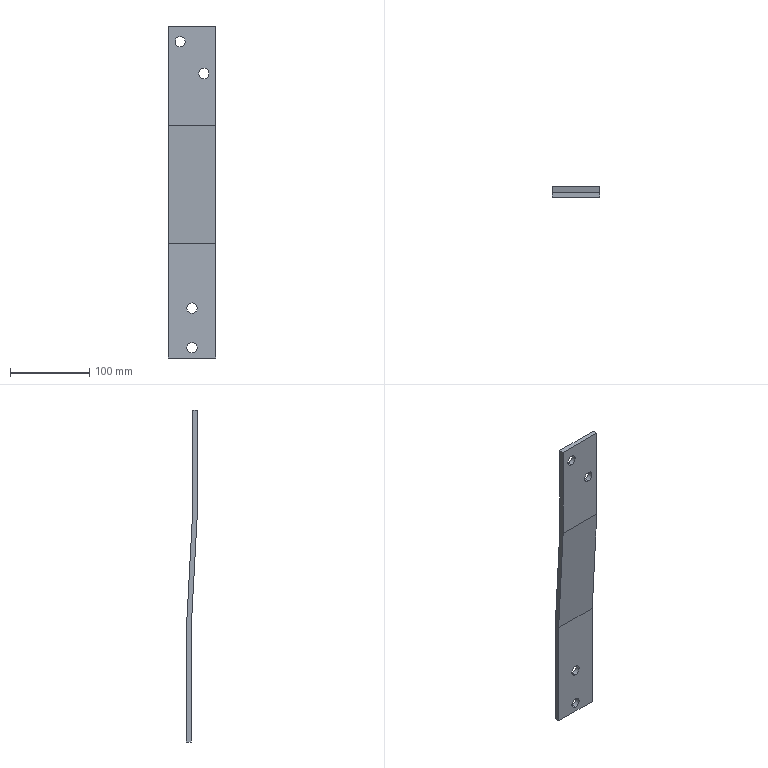Part | SolidWorks | features BaseBody 1 | 1 solid | 18 faces | box 60 x 14 x 419 mm | volume 147654 mm3 | plane 10 | cylinder 8 | commonest cylinder face diameters 13 x8
STEP:
#1=CARTESIAN_POINT('',(756.946,-3480.473,1580.471));
#2=VERTEX_POINT('',#1);
#3=CARTESIAN_POINT('',(756.946,-3480.473,1567.471));
#4=VERTEX_POINT('',#3);
#5=CARTESIAN_POINT('',(756.946,-3480.473,1573.971));
#6=DIRECTION('',(0.,-1.,0.));
#7=DIRECTION('',(0.,0.,-1.));
#8=AXIS2_PLACEMENT_3D('',#5,#6,#7);
#9=CIRCLE('',#8,6.5);
#10=EDGE_CURVE('',#2,#4,#9,.T.);
#11=ORIENTED_EDGE('',*,*,#10,.F.);
#12=CARTESIAN_POINT('',(756.946,-3486.473,1580.471));
#13=VERTEX_POINT('',#12);
#14=CARTESIAN_POINT('',(756.946,-3491.9,1580.471));
#15=DIRECTION('',(0.,-1.,0.));
#16=VECTOR('',#15,1000.);
#17=LINE('',#14,#16);
#18=EDGE_CURVE('',#2,#13,#17,.T.);
#19=ORIENTED_EDGE('',*,*,#18,.T.);
#20=CARTESIAN_POINT('',(756.946,-3486.473,1567.471));
#21=VERTEX_POINT('',#20);
#22=CARTESIAN_POINT('',(756.946,-3486.473,1573.971));
#23=DIRECTION('',(0.,1.,0.));
#24=DIRECTION('',(0.,0.,-1.));
#25=AXIS2_PLACEMENT_3D('',#22,#23,#24);
#26=CIRCLE('',#25,6.5);
#27=EDGE_CURVE('',#21,#13,#26,.T.);
#28=ORIENTED_EDGE('',*,*,#27,.F.);
#29=CARTESIAN_POINT('',(756.946,-3491.9,1567.471));
#30=DIRECTION('',(0.,-1.,0.));
#31=VECTOR('',#30,1000.);
#32=LINE('',#29,#31);
#33=EDGE_CURVE('',#4,#21,#32,.T.);
#34=ORIENTED_EDGE('',*,*,#33,.F.);
#35=EDGE_LOOP('',(#11,#19,#28,#34));
#36=FACE_OUTER_BOUND('',#35,.T.);
#37=CARTESIAN_POINT('',(756.946,-3491.9,1573.971));
#38=DIRECTION('',(0.,-1.,0.));
#39=DIRECTION('',(0.,0.,-1.));
#40=AXIS2_PLACEMENT_3D('',#37,#38,#39);
#41=CYLINDRICAL_SURFACE('',#40,6.5);
#42=ADVANCED_FACE('',(#36),#41,.F.);
#43=CARTESIAN_POINT('',(756.946,-3480.473,1530.471));
#44=VERTEX_POINT('',#43);
#45=CARTESIAN_POINT('',(756.946,-3480.473,1517.471));
#46=VERTEX_POINT('',#45);
#47=CARTESIAN_POINT('',(756.946,-3480.473,1523.971));
#48=DIRECTION('',(0.,-1.,0.));
#49=DIRECTION('',(0.,0.,-1.));
#50=AXIS2_PLACEMENT_3D('',#47,#48,#49);
#51=CIRCLE('',#50,6.5);
#52=EDGE_CURVE('',#44,#46,#51,.T.);
#53=ORIENTED_EDGE('',*,*,#52,.F.);
#54=CARTESIAN_POINT('',(756.946,-3486.473,1530.471));
#55=VERTEX_POINT('',#54);
#56=CARTESIAN_POINT('',(756.946,-3491.9,1530.471));
#57=DIRECTION('',(0.,-1.,0.));
#58=VECTOR('',#57,1000.);
#59=LINE('',#56,#58);
#60=EDGE_CURVE('',#44,#55,#59,.T.);
#61=ORIENTED_EDGE('',*,*,#60,.T.);
#62=CARTESIAN_POINT('',(756.946,-3486.473,1517.471));
#63=VERTEX_POINT('',#62);
#64=CARTESIAN_POINT('',(756.946,-3486.473,1523.971));
#65=DIRECTION('',(0.,1.,0.));
#66=DIRECTION('',(0.,0.,-1.));
#67=AXIS2_PLACEMENT_3D('',#64,#65,#66);
#68=CIRCLE('',#67,6.5);
#69=EDGE_CURVE('',#63,#55,#68,.T.);
#70=ORIENTED_EDGE('',*,*,#69,.F.);
#71=CARTESIAN_POINT('',(756.946,-3491.9,1517.471));
#72=DIRECTION('',(0.,-1.,0.));
#73=VECTOR('',#72,1000.);
#74=LINE('',#71,#73);
#75=EDGE_CURVE('',#46,#63,#74,.T.);
#76=ORIENTED_EDGE('',*,*,#75,.F.);
#77=EDGE_LOOP('',(#53,#61,#70,#76));
#78=FACE_OUTER_BOUND('',#77,.T.);
#79=CARTESIAN_POINT('',(756.946,-3491.9,1523.971));
#80=DIRECTION('',(0.,-1.,0.));
#81=DIRECTION('',(0.,0.,-1.));
#82=AXIS2_PLACEMENT_3D('',#79,#80,#81);
#83=CYLINDRICAL_SURFACE('',#82,6.5);
#84=ADVANCED_FACE('',(#78),#83,.F.);
#85=CARTESIAN_POINT('',(741.946,-3488.473,1916.471));
#86=VERTEX_POINT('',#85);
#87=CARTESIAN_POINT('',(741.946,-3488.473,1903.471));
#88=VERTEX_POINT('',#87);
#89=CARTESIAN_POINT('',(741.946,-3488.473,1909.971));
#90=DIRECTION('',(0.,-1.,0.));
#91=DIRECTION('',(0.,0.,-1.));
#92=AXIS2_PLACEMENT_3D('',#89,#90,#91);
#93=CIRCLE('',#92,6.5);
#94=EDGE_CURVE('',#86,#88,#93,.T.);
#95=ORIENTED_EDGE('',*,*,#94,.F.);
#96=CARTESIAN_POINT('',(741.946,-3494.473,1916.471));
#97=VERTEX_POINT('',#96);
#98=CARTESIAN_POINT('',(741.946,-3489.856,1916.471));
#99=DIRECTION('',(0.,-1.,0.));
#100=VECTOR('',#99,1000.);
#101=LINE('',#98,#100);
#102=EDGE_CURVE('',#86,#97,#101,.T.);
#103=ORIENTED_EDGE('',*,*,#102,.T.);
#104=CARTESIAN_POINT('',(741.946,-3494.473,1903.471));
#105=VERTEX_POINT('',#104);
#106=CARTESIAN_POINT('',(741.946,-3494.473,1909.971));
#107=DIRECTION('',(0.,1.,0.));
#108=DIRECTION('',(0.,0.,-1.));
#109=AXIS2_PLACEMENT_3D('',#106,#107,#108);
#110=CIRCLE('',#109,6.5);
#111=EDGE_CURVE('',#105,#97,#110,.T.);
#112=ORIENTED_EDGE('',*,*,#111,.F.);
#113=CARTESIAN_POINT('',(741.946,-3489.856,1903.471));
#114=DIRECTION('',(0.,-1.,0.));
#115=VECTOR('',#114,1000.);
#116=LINE('',#113,#115);
#117=EDGE_CURVE('',#88,#105,#116,.T.);
#118=ORIENTED_EDGE('',*,*,#117,.F.);
#119=EDGE_LOOP('',(#95,#103,#112,#118));
#120=FACE_OUTER_BOUND('',#119,.T.);
#121=CARTESIAN_POINT('',(741.946,-3489.856,1909.971));
#122=DIRECTION('',(0.,-1.,0.));
#123=DIRECTION('',(0.,0.,-1.));
#124=AXIS2_PLACEMENT_3D('',#121,#122,#123);
#125=CYLINDRICAL_SURFACE('',#124,6.5);
#126=ADVANCED_FACE('',(#120),#125,.F.);
#127=CARTESIAN_POINT('',(771.946,-3488.473,1876.471));
#128=VERTEX_POINT('',#127);
#129=CARTESIAN_POINT('',(771.946,-3488.473,1863.471));
#130=VERTEX_POINT('',#129);
#131=CARTESIAN_POINT('',(771.946,-3488.473,1869.971));
#132=DIRECTION('',(0.,-1.,0.));
#133=DIRECTION('',(0.,0.,-1.));
#134=AXIS2_PLACEMENT_3D('',#131,#132,#133);
#135=CIRCLE('',#134,6.5);
#136=EDGE_CURVE('',#128,#130,#135,.T.);
#137=ORIENTED_EDGE('',*,*,#136,.F.);
#138=CARTESIAN_POINT('',(771.946,-3494.473,1876.471));
#139=VERTEX_POINT('',#138);
#140=CARTESIAN_POINT('',(771.946,-3487.265,1876.471));
#141=DIRECTION('',(0.,-1.,0.));
#142=VECTOR('',#141,1000.);
#143=LINE('',#140,#142);
#144=EDGE_CURVE('',#128,#139,#143,.T.);
#145=ORIENTED_EDGE('',*,*,#144,.T.);
#146=CARTESIAN_POINT('',(771.946,-3494.473,1863.471));
#147=VERTEX_POINT('',#146);
#148=CARTESIAN_POINT('',(771.946,-3494.473,1869.971));
#149=DIRECTION('',(0.,1.,0.));
#150=DIRECTION('',(0.,0.,-1.));
#151=AXIS2_PLACEMENT_3D('',#148,#149,#150);
#152=CIRCLE('',#151,6.5);
#153=EDGE_CURVE('',#147,#139,#152,.T.);
#154=ORIENTED_EDGE('',*,*,#153,.F.);
#155=CARTESIAN_POINT('',(771.946,-3487.265,1863.471));
#156=DIRECTION('',(0.,-1.,0.));
#157=VECTOR('',#156,1000.);
#158=LINE('',#155,#157);
#159=EDGE_CURVE('',#130,#147,#158,.T.);
#160=ORIENTED_EDGE('',*,*,#159,.F.);
#161=EDGE_LOOP('',(#137,#145,#154,#160));
#162=FACE_OUTER_BOUND('',#161,.T.);
#163=CARTESIAN_POINT('',(771.946,-3487.265,1869.971));
#164=DIRECTION('',(0.,-1.,0.));
#165=DIRECTION('',(0.,0.,-1.));
#166=AXIS2_PLACEMENT_3D('',#163,#164,#165);
#167=CYLINDRICAL_SURFACE('',#166,6.5);
#168=ADVANCED_FACE('',(#162),#167,.F.);
#169=CARTESIAN_POINT('',(786.946,-3488.473,1804.971));
#170=VERTEX_POINT('',#169);
#171=CARTESIAN_POINT('',(786.946,-3480.473,1654.971));
#172=VERTEX_POINT('',#171);
#173=CARTESIAN_POINT('',(786.946,-3480.473,1654.971));
#174=DIRECTION('',(0.,0.05326,-0.9986));
#175=VECTOR('',#174,1000.);
#176=LINE('',#173,#175);
#177=EDGE_CURVE('',#170,#172,#176,.T.);
#178=ORIENTED_EDGE('',*,*,#177,.T.);
#179=CARTESIAN_POINT('',(726.946,-3480.473,1654.971));
#180=VERTEX_POINT('',#179);
#181=CARTESIAN_POINT('',(786.946,-3480.473,1654.971));
#182=DIRECTION('',(-1.,0.,0.));
#183=VECTOR('',#182,1000.);
#184=LINE('',#181,#183);
#185=EDGE_CURVE('',#172,#180,#184,.T.);
#186=ORIENTED_EDGE('',*,*,#185,.T.);
#187=CARTESIAN_POINT('',(726.946,-3488.473,1804.971));
#188=VERTEX_POINT('',#187);
#189=CARTESIAN_POINT('',(726.946,-3480.473,1654.971));
#190=DIRECTION('',(0.,-0.05326,0.9986));
#191=VECTOR('',#190,1000.);
#192=LINE('',#189,#191);
#193=EDGE_CURVE('',#180,#188,#192,.T.);
#194=ORIENTED_EDGE('',*,*,#193,.T.);
#195=CARTESIAN_POINT('',(786.946,-3488.473,1804.971));
#196=DIRECTION('',(1.,0.,0.));
#197=VECTOR('',#196,1000.);
#198=LINE('',#195,#197);
#199=EDGE_CURVE('',#188,#170,#198,.T.);
#200=ORIENTED_EDGE('',*,*,#199,.T.);
#201=EDGE_LOOP('',(#178,#186,#194,#200));
#202=FACE_OUTER_BOUND('',#201,.T.);
#203=CARTESIAN_POINT('',(786.946,-3480.473,1654.971));
#204=DIRECTION('',(0.,0.9986,0.05326));
#205=DIRECTION('',(0.,-0.05326,0.9986));
#206=AXIS2_PLACEMENT_3D('',#203,#204,#205);
#207=PLANE('',#206);
#208=ADVANCED_FACE('',(#202),#207,.T.);
#209=CARTESIAN_POINT('',(786.946,-3480.473,1510.971));
#210=VERTEX_POINT('',#209);
#211=CARTESIAN_POINT('',(786.946,-3480.473,1510.971));
#212=DIRECTION('',(0.,0.,-1.));
#213=VECTOR('',#212,1000.);
#214=LINE('',#211,#213);
#215=EDGE_CURVE('',#172,#210,#214,.T.);
#216=ORIENTED_EDGE('',*,*,#215,.T.);
#217=CARTESIAN_POINT('',(726.946,-3480.473,1510.971));
#218=VERTEX_POINT('',#217);
#219=CARTESIAN_POINT('',(786.946,-3480.473,1510.971));
#220=DIRECTION('',(-1.,0.,0.));
#221=VECTOR('',#220,1000.);
#222=LINE('',#219,#221);
#223=EDGE_CURVE('',#210,#218,#222,.T.);
#224=ORIENTED_EDGE('',*,*,#223,.T.);
#225=CARTESIAN_POINT('',(726.946,-3480.473,1510.971));
#226=DIRECTION('',(0.,0.,1.));
#227=VECTOR('',#226,1000.);
#228=LINE('',#225,#227);
#229=EDGE_CURVE('',#218,#180,#228,.T.);
#230=ORIENTED_EDGE('',*,*,#229,.T.);
#231=ORIENTED_EDGE('',*,*,#185,.F.);
#232=EDGE_LOOP('',(#216,#224,#230,#231));
#233=FACE_OUTER_BOUND('',#232,.T.);
#234=CARTESIAN_POINT('',(756.946,-3480.473,1573.971));
#235=DIRECTION('',(0.,-1.,0.));
#236=DIRECTION('',(0.,0.,-1.));
#237=AXIS2_PLACEMENT_3D('',#234,#235,#236);
#238=CIRCLE('',#237,6.5);
#239=EDGE_CURVE('',#4,#2,#238,.T.);
#240=ORIENTED_EDGE('',*,*,#239,.T.);
#241=ORIENTED_EDGE('',*,*,#10,.T.);
#242=EDGE_LOOP('',(#240,#241));
#243=FACE_BOUND('',#242,.T.);
#244=CARTESIAN_POINT('',(756.946,-3480.473,1523.971));
#245=DIRECTION('',(0.,-1.,0.));
#246=DIRECTION('',(0.,0.,-1.));
#247=AXIS2_PLACEMENT_3D('',#244,#245,#246);
#248=CIRCLE('',#247,6.5);
#249=EDGE_CURVE('',#46,#44,#248,.T.);
#250=ORIENTED_EDGE('',*,*,#249,.T.);
#251=ORIENTED_EDGE('',*,*,#52,.T.);
#252=EDGE_LOOP('',(#250,#251));
#253=FACE_BOUND('',#252,.T.);
#254=CARTESIAN_POINT('',(786.946,-3480.473,1510.971));
#255=DIRECTION('',(0.,1.,0.));
#256=DIRECTION('',(0.,0.,1.));
#257=AXIS2_PLACEMENT_3D('',#254,#255,#256);
#258=PLANE('',#257);
#259=ADVANCED_FACE('',(#233,#243,#253),#258,.T.);
#260=CARTESIAN_POINT('',(786.946,-3494.473,1804.971));
#261=VERTEX_POINT('',#260);
#262=CARTESIAN_POINT('',(786.946,-3486.473,1654.971));
#263=VERTEX_POINT('',#262);
#264=CARTESIAN_POINT('',(786.946,-3494.473,1804.971));
#265=DIRECTION('',(0.,0.05326,-0.9986));
#266=VECTOR('',#265,1000.);
#267=LINE('',#264,#266);
#268=EDGE_CURVE('',#261,#263,#267,.T.);
#269=ORIENTED_EDGE('',*,*,#268,.T.);
#270=CARTESIAN_POINT('',(786.946,-3486.473,1510.971));
#271=VERTEX_POINT('',#270);
#272=CARTESIAN_POINT('',(786.946,-3486.473,1707.983));
#273=DIRECTION('',(0.,0.,-1.));
#274=VECTOR('',#273,1000.);
#275=LINE('',#272,#274);
#276=EDGE_CURVE('',#263,#271,#275,.T.);
#277=ORIENTED_EDGE('',*,*,#276,.T.);
#278=CARTESIAN_POINT('',(786.946,-3487.033,1510.971));
#279=DIRECTION('',(0.,1.,0.));
#280=VECTOR('',#279,1000.);
#281=LINE('',#278,#280);
#282=EDGE_CURVE('',#271,#210,#281,.T.);
#283=ORIENTED_EDGE('',*,*,#282,.T.);
#284=ORIENTED_EDGE('',*,*,#215,.F.);
#285=ORIENTED_EDGE('',*,*,#177,.F.);
#286=CARTESIAN_POINT('',(786.946,-3488.473,1929.971));
#287=VERTEX_POINT('',#286);
#288=CARTESIAN_POINT('',(786.946,-3488.473,1707.983));
#289=DIRECTION('',(0.,0.,1.));
#290=VECTOR('',#289,1000.);
#291=LINE('',#288,#290);
#292=EDGE_CURVE('',#170,#287,#291,.T.);
#293=ORIENTED_EDGE('',*,*,#292,.T.);
#294=CARTESIAN_POINT('',(786.946,-3494.473,1929.971));
#295=VERTEX_POINT('',#294);
#296=CARTESIAN_POINT('',(786.946,-3487.033,1929.971));
#297=DIRECTION('',(0.,-1.,0.));
#298=VECTOR('',#297,1000.);
#299=LINE('',#296,#298);
#300=EDGE_CURVE('',#287,#295,#299,.T.);
#301=ORIENTED_EDGE('',*,*,#300,.T.);
#302=CARTESIAN_POINT('',(786.946,-3494.473,1707.983));
#303=DIRECTION('',(0.,0.,-1.));
#304=VECTOR('',#303,1000.);
#305=LINE('',#302,#304);
#306=EDGE_CURVE('',#295,#261,#305,.T.);
#307=ORIENTED_EDGE('',*,*,#306,.T.);
#308=EDGE_LOOP('',(#269,#277,#283,#284,#285,#293,#301,#307));
#309=FACE_OUTER_BOUND('',#308,.T.);
#310=CARTESIAN_POINT('',(786.946,-3487.033,1707.983));
#311=DIRECTION('',(1.,0.,0.));
#312=DIRECTION('',(0.,0.,-1.));
#313=AXIS2_PLACEMENT_3D('',#310,#311,#312);
#314=PLANE('',#313);
#315=ADVANCED_FACE('',(#309),#314,.T.);
#316=ORIENTED_EDGE('',*,*,#292,.F.);
#317=ORIENTED_EDGE('',*,*,#199,.F.);
#318=CARTESIAN_POINT('',(726.946,-3488.473,1929.971));
#319=VERTEX_POINT('',#318);
#320=CARTESIAN_POINT('',(726.946,-3488.473,1804.971));
#321=DIRECTION('',(0.,0.,1.));
#322=VECTOR('',#321,1000.);
#323=LINE('',#320,#322);
#324=EDGE_CURVE('',#188,#319,#323,.T.);
#325=ORIENTED_EDGE('',*,*,#324,.T.);
#326=CARTESIAN_POINT('',(786.946,-3488.473,1929.971));
#327=DIRECTION('',(1.,0.,0.));
#328=VECTOR('',#327,1000.);
#329=LINE('',#326,#328);
#330=EDGE_CURVE('',#319,#287,#329,.T.);
#331=ORIENTED_EDGE('',*,*,#330,.T.);
#332=EDGE_LOOP('',(#316,#317,#325,#331));
#333=FACE_OUTER_BOUND('',#332,.T.);
#334=CARTESIAN_POINT('',(741.946,-3488.473,1909.971));
#335=DIRECTION('',(0.,-1.,0.));
#336=DIRECTION('',(0.,0.,-1.));
#337=AXIS2_PLACEMENT_3D('',#334,#335,#336);
#338=CIRCLE('',#337,6.5);
#339=EDGE_CURVE('',#88,#86,#338,.T.);
#340=ORIENTED_EDGE('',*,*,#339,.T.);
#341=ORIENTED_EDGE('',*,*,#94,.T.);
#342=EDGE_LOOP('',(#340,#341));
#343=FACE_BOUND('',#342,.T.);
#344=CARTESIAN_POINT('',(771.946,-3488.473,1869.971));
#345=DIRECTION('',(0.,-1.,0.));
#346=DIRECTION('',(0.,0.,-1.));
#347=AXIS2_PLACEMENT_3D('',#344,#345,#346);
#348=CIRCLE('',#347,6.5);
#349=EDGE_CURVE('',#130,#128,#348,.T.);
#350=ORIENTED_EDGE('',*,*,#349,.T.);
#351=ORIENTED_EDGE('',*,*,#136,.T.);
#352=EDGE_LOOP('',(#350,#351));
#353=FACE_BOUND('',#352,.T.);
#354=CARTESIAN_POINT('',(786.946,-3488.473,1804.971));
#355=DIRECTION('',(0.,1.,0.));
#356=DIRECTION('',(0.,0.,1.));
#357=AXIS2_PLACEMENT_3D('',#354,#355,#356);
#358=PLANE('',#357);
#359=ADVANCED_FACE('',(#333,#343,#353),#358,.T.);
#360=CARTESIAN_POINT('',(726.946,-3486.473,1510.971));
#361=VERTEX_POINT('',#360);
#362=CARTESIAN_POINT('',(726.946,-3487.033,1510.971));
#363=DIRECTION('',(0.,1.,0.));
#364=VECTOR('',#363,1000.);
#365=LINE('',#362,#364);
#366=EDGE_CURVE('',#361,#218,#365,.T.);
#367=ORIENTED_EDGE('',*,*,#366,.F.);
#368=CARTESIAN_POINT('',(726.946,-3486.473,1654.971));
#369=VERTEX_POINT('',#368);
#370=CARTESIAN_POINT('',(726.946,-3486.473,1707.983));
#371=DIRECTION('',(0.,0.,-1.));
#372=VECTOR('',#371,1000.);
#373=LINE('',#370,#372);
#374=EDGE_CURVE('',#369,#361,#373,.T.);
#375=ORIENTED_EDGE('',*,*,#374,.F.);
#376=CARTESIAN_POINT('',(726.946,-3494.473,1804.971));
#377=VERTEX_POINT('',#376);
#378=CARTESIAN_POINT('',(726.946,-3494.473,1804.971));
#379=DIRECTION('',(0.,0.05326,-0.9986));
#380=VECTOR('',#379,1000.);
#381=LINE('',#378,#380);
#382=EDGE_CURVE('',#377,#369,#381,.T.);
#383=ORIENTED_EDGE('',*,*,#382,.F.);
#384=CARTESIAN_POINT('',(726.946,-3494.473,1929.971));
#385=VERTEX_POINT('',#384);
#386=CARTESIAN_POINT('',(726.946,-3494.473,1707.983));
#387=DIRECTION('',(0.,0.,-1.));
#388=VECTOR('',#387,1000.);
#389=LINE('',#386,#388);
#390=EDGE_CURVE('',#385,#377,#389,.T.);
#391=ORIENTED_EDGE('',*,*,#390,.F.);
#392=CARTESIAN_POINT('',(726.946,-3487.033,1929.971));
#393=DIRECTION('',(0.,-1.,0.));
#394=VECTOR('',#393,1000.);
#395=LINE('',#392,#394);
#396=EDGE_CURVE('',#319,#385,#395,.T.);
#397=ORIENTED_EDGE('',*,*,#396,.F.);
#398=ORIENTED_EDGE('',*,*,#324,.F.);
#399=ORIENTED_EDGE('',*,*,#193,.F.);
#400=ORIENTED_EDGE('',*,*,#229,.F.);
#401=EDGE_LOOP('',(#367,#375,#383,#391,#397,#398,#399,#400));
#402=FACE_OUTER_BOUND('',#401,.T.);
#403=CARTESIAN_POINT('',(726.946,-3487.033,1707.983));
#404=DIRECTION('',(1.,0.,0.));
#405=DIRECTION('',(0.,0.,-1.));
#406=AXIS2_PLACEMENT_3D('',#403,#404,#405);
#407=PLANE('',#406);
#408=ADVANCED_FACE('',(#402),#407,.F.);
#409=ORIENTED_EDGE('',*,*,#282,.F.);
#410=CARTESIAN_POINT('',(786.946,-3486.473,1510.971));
#411=DIRECTION('',(-1.,0.,0.));
#412=VECTOR('',#411,1000.);
#413=LINE('',#410,#412);
#414=EDGE_CURVE('',#271,#361,#413,.T.);
#415=ORIENTED_EDGE('',*,*,#414,.T.);
#416=ORIENTED_EDGE('',*,*,#366,.T.);
#417=ORIENTED_EDGE('',*,*,#223,.F.);
#418=EDGE_LOOP('',(#409,#415,#416,#417));
#419=FACE_OUTER_BOUND('',#418,.T.);
#420=CARTESIAN_POINT('',(786.946,-3486.473,1510.971));
#421=DIRECTION('',(0.,0.,-1.));
#422=DIRECTION('',(-1.,0.,0.));
#423=AXIS2_PLACEMENT_3D('',#420,#421,#422);
#424=PLANE('',#423);
#425=ADVANCED_FACE('',(#419),#424,.T.);
#426=ORIENTED_EDGE('',*,*,#18,.F.);
#427=ORIENTED_EDGE('',*,*,#239,.F.);
#428=ORIENTED_EDGE('',*,*,#33,.T.);
#429=CARTESIAN_POINT('',(756.946,-3486.473,1573.971));
#430=DIRECTION('',(0.,1.,0.));
#431=DIRECTION('',(0.,0.,-1.));
#432=AXIS2_PLACEMENT_3D('',#429,#430,#431);
#433=CIRCLE('',#432,6.5);
#434=EDGE_CURVE('',#13,#21,#433,.T.);
#435=ORIENTED_EDGE('',*,*,#434,.F.);
#436=EDGE_LOOP('',(#426,#427,#428,#435));
#437=FACE_OUTER_BOUND('',#436,.T.);
#438=CARTESIAN_POINT('',(756.946,-3491.9,1573.971));
#439=DIRECTION('',(0.,-1.,0.));
#440=DIRECTION('',(0.,0.,-1.));
#441=AXIS2_PLACEMENT_3D('',#438,#439,#440);
#442=CYLINDRICAL_SURFACE('',#441,6.5);
#443=ADVANCED_FACE('',(#437),#442,.F.);
#444=ORIENTED_EDGE('',*,*,#60,.F.);
#445=ORIENTED_EDGE('',*,*,#249,.F.);
#446=ORIENTED_EDGE('',*,*,#75,.T.);
#447=CARTESIAN_POINT('',(756.946,-3486.473,1523.971));
#448=DIRECTION('',(0.,1.,0.));
#449=DIRECTION('',(0.,0.,-1.));
#450=AXIS2_PLACEMENT_3D('',#447,#448,#449);
#451=CIRCLE('',#450,6.5);
#452=EDGE_CURVE('',#55,#63,#451,.T.);
#453=ORIENTED_EDGE('',*,*,#452,.F.);
#454=EDGE_LOOP('',(#444,#445,#446,#453));
#455=FACE_OUTER_BOUND('',#454,.T.);
#456=CARTESIAN_POINT('',(756.946,-3491.9,1523.971));
#457=DIRECTION('',(0.,-1.,0.));
#458=DIRECTION('',(0.,0.,-1.));
#459=AXIS2_PLACEMENT_3D('',#456,#457,#458);
#460=CYLINDRICAL_SURFACE('',#459,6.5);
#461=ADVANCED_FACE('',(#455),#460,.F.);
#462=ORIENTED_EDGE('',*,*,#276,.F.);
#463=CARTESIAN_POINT('',(786.946,-3486.473,1654.971));
#464=DIRECTION('',(-1.,0.,0.));
#465=VECTOR('',#464,1000.);
#466=LINE('',#463,#465);
#467=EDGE_CURVE('',#263,#369,#466,.T.);
#468=ORIENTED_EDGE('',*,*,#467,.T.);
#469=ORIENTED_EDGE('',*,*,#374,.T.);
#470=ORIENTED_EDGE('',*,*,#414,.F.);
#471=EDGE_LOOP('',(#462,#468,#469,#470));
#472=FACE_OUTER_BOUND('',#471,.T.);
#473=ORIENTED_EDGE('',*,*,#27,.T.);
#474=ORIENTED_EDGE('',*,*,#434,.T.);
#475=EDGE_LOOP('',(#473,#474));
#476=FACE_BOUND('',#475,.T.);
#477=ORIENTED_EDGE('',*,*,#69,.T.);
#478=ORIENTED_EDGE('',*,*,#452,.T.);
#479=EDGE_LOOP('',(#477,#478));
#480=FACE_BOUND('',#479,.T.);
#481=CARTESIAN_POINT('',(786.946,-3486.473,1654.971));
#482=DIRECTION('',(0.,-1.,0.));
#483=DIRECTION('',(0.,0.,-1.));
#484=AXIS2_PLACEMENT_3D('',#481,#482,#483);
#485=PLANE('',#484);
#486=ADVANCED_FACE('',(#472,#476,#480),#485,.T.);
#487=ORIENTED_EDGE('',*,*,#268,.F.);
#488=CARTESIAN_POINT('',(786.946,-3494.473,1804.971));
#489=DIRECTION('',(-1.,0.,0.));
#490=VECTOR('',#489,1000.);
#491=LINE('',#488,#490);
#492=EDGE_CURVE('',#261,#377,#491,.T.);
#493=ORIENTED_EDGE('',*,*,#492,.T.);
#494=ORIENTED_EDGE('',*,*,#382,.T.);
#495=ORIENTED_EDGE('',*,*,#467,.F.);
#496=EDGE_LOOP('',(#487,#493,#494,#495));
#497=FACE_OUTER_BOUND('',#496,.T.);
#498=CARTESIAN_POINT('',(786.946,-3494.473,1804.971));
#499=DIRECTION('',(0.,-0.9986,-0.05326));
#500=DIRECTION('',(0.,0.05326,-0.9986));
#501=AXIS2_PLACEMENT_3D('',#498,#499,#500);
#502=PLANE('',#501);
#503=ADVANCED_FACE('',(#497),#502,.T.);
#504=ORIENTED_EDGE('',*,*,#306,.F.);
#505=CARTESIAN_POINT('',(786.946,-3494.473,1929.971));
#506=DIRECTION('',(-1.,0.,0.));
#507=VECTOR('',#506,1000.);
#508=LINE('',#505,#507);
#509=EDGE_CURVE('',#295,#385,#508,.T.);
#510=ORIENTED_EDGE('',*,*,#509,.T.);
#511=ORIENTED_EDGE('',*,*,#390,.T.);
#512=ORIENTED_EDGE('',*,*,#492,.F.);
#513=EDGE_LOOP('',(#504,#510,#511,#512));
#514=FACE_OUTER_BOUND('',#513,.T.);
#515=ORIENTED_EDGE('',*,*,#111,.T.);
#516=CARTESIAN_POINT('',(741.946,-3494.473,1909.971));
#517=DIRECTION('',(0.,1.,0.));
#518=DIRECTION('',(0.,0.,-1.));
#519=AXIS2_PLACEMENT_3D('',#516,#517,#518);
#520=CIRCLE('',#519,6.5);
#521=EDGE_CURVE('',#97,#105,#520,.T.);
#522=ORIENTED_EDGE('',*,*,#521,.T.);
#523=EDGE_LOOP('',(#515,#522));
#524=FACE_BOUND('',#523,.T.);
#525=ORIENTED_EDGE('',*,*,#153,.T.);
#526=CARTESIAN_POINT('',(771.946,-3494.473,1869.971));
#527=DIRECTION('',(0.,1.,0.));
#528=DIRECTION('',(0.,0.,-1.));
#529=AXIS2_PLACEMENT_3D('',#526,#527,#528);
#530=CIRCLE('',#529,6.5);
#531=EDGE_CURVE('',#139,#147,#530,.T.);
#532=ORIENTED_EDGE('',*,*,#531,.T.);
#533=EDGE_LOOP('',(#525,#532));
#534=FACE_BOUND('',#533,.T.);
#535=CARTESIAN_POINT('',(786.946,-3494.473,1904.971));
#536=DIRECTION('',(0.,-1.,0.));
#537=DIRECTION('',(0.,0.,-1.));
#538=AXIS2_PLACEMENT_3D('',#535,#536,#537);
#539=PLANE('',#538);
#540=ADVANCED_FACE('',(#514,#524,#534),#539,.T.);
#541=ORIENTED_EDGE('',*,*,#300,.F.);
#542=ORIENTED_EDGE('',*,*,#330,.F.);
#543=ORIENTED_EDGE('',*,*,#396,.T.);
#544=ORIENTED_EDGE('',*,*,#509,.F.);
#545=EDGE_LOOP('',(#541,#542,#543,#544));
#546=FACE_OUTER_BOUND('',#545,.T.);
#547=CARTESIAN_POINT('',(786.946,-3488.473,1929.971));
#548=DIRECTION('',(0.,0.,1.));
#549=DIRECTION('',(1.,0.,0.));
#550=AXIS2_PLACEMENT_3D('',#547,#548,#549);
#551=PLANE('',#550);
#552=ADVANCED_FACE('',(#546),#551,.T.);
#553=ORIENTED_EDGE('',*,*,#102,.F.);
#554=ORIENTED_EDGE('',*,*,#339,.F.);
#555=ORIENTED_EDGE('',*,*,#117,.T.);
#556=ORIENTED_EDGE('',*,*,#521,.F.);
#557=EDGE_LOOP('',(#553,#554,#555,#556));
#558=FACE_OUTER_BOUND('',#557,.T.);
#559=CARTESIAN_POINT('',(741.946,-3489.856,1909.971));
#560=DIRECTION('',(0.,-1.,0.));
#561=DIRECTION('',(0.,0.,-1.));
#562=AXIS2_PLACEMENT_3D('',#559,#560,#561);
#563=CYLINDRICAL_SURFACE('',#562,6.5);
#564=ADVANCED_FACE('',(#558),#563,.F.);
#565=ORIENTED_EDGE('',*,*,#144,.F.);
#566=ORIENTED_EDGE('',*,*,#349,.F.);
#567=ORIENTED_EDGE('',*,*,#159,.T.);
#568=ORIENTED_EDGE('',*,*,#531,.F.);
#569=EDGE_LOOP('',(#565,#566,#567,#568));
#570=FACE_OUTER_BOUND('',#569,.T.);
#571=CARTESIAN_POINT('',(771.946,-3487.265,1869.971));
#572=DIRECTION('',(0.,-1.,0.));
#573=DIRECTION('',(0.,0.,-1.));
#574=AXIS2_PLACEMENT_3D('',#571,#572,#573);
#575=CYLINDRICAL_SURFACE('',#574,6.5);
#576=ADVANCED_FACE('',(#570),#575,.F.);
#577=CLOSED_SHELL('',(#42,#84,#126,#168,#208,#259,#315,#359,#408,#425,#443,#461,#486,#503,#540,#552,#564,#576));
#578=MANIFOLD_SOLID_BREP('',#577);
#579=CARTESIAN_POINT('',(0.,0.,0.));
#580=DIRECTION('',(0.,0.,1.));
#581=DIRECTION('',(1.,0.,0.));
#582=AXIS2_PLACEMENT_3D('',#579,#580,#581);
#583=(LENGTH_UNIT()NAMED_UNIT(*)SI_UNIT(.MILLI.,.METRE.));
#584=UNCERTAINTY_MEASURE_WITH_UNIT(LENGTH_MEASURE(0.00001),#583,'','');
#585=(NAMED_UNIT(*)PLANE_ANGLE_UNIT()SI_UNIT($,.RADIAN.));
#586=(NAMED_UNIT(*)SI_UNIT($,.STERADIAN.)SOLID_ANGLE_UNIT());
#587=(GEOMETRIC_REPRESENTATION_CONTEXT(3)GLOBAL_UNCERTAINTY_ASSIGNED_CONTEXT((#584))GLOBAL_UNIT_ASSIGNED_CONTEXT((#583,#585,#586))REPRESENTATION_CONTEXT('',''));
#588=ADVANCED_BREP_SHAPE_REPRESENTATION('',(#578,#582),#587);